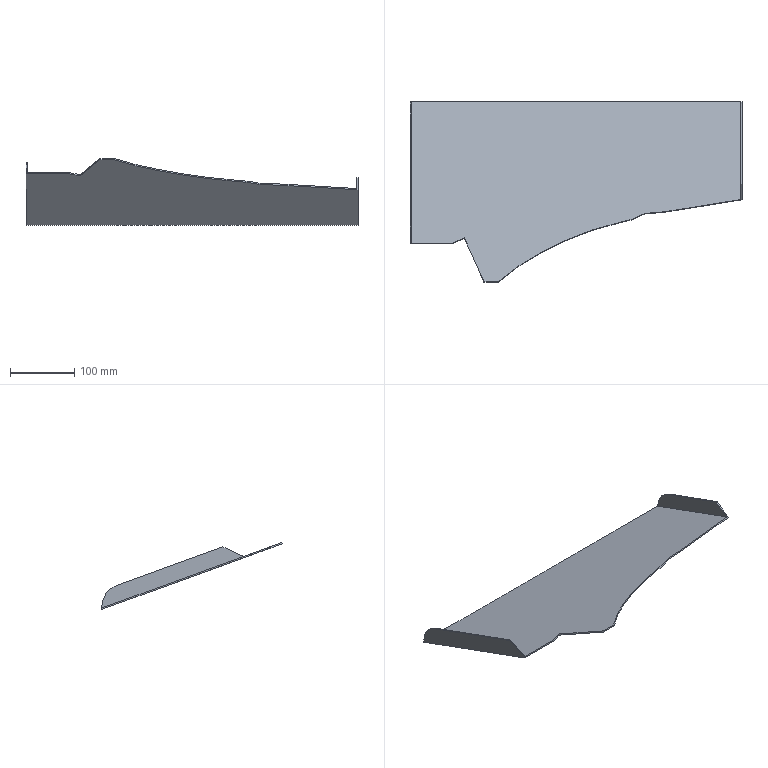Part | NX | features solid 2 | 1 solid | 18 faces | box 515 x 279.899 x 103.754 mm | volume 243833 mm3 | plane 15 | cylinder 2 | spline 1 | commonest cylinder face diameters 70 x2